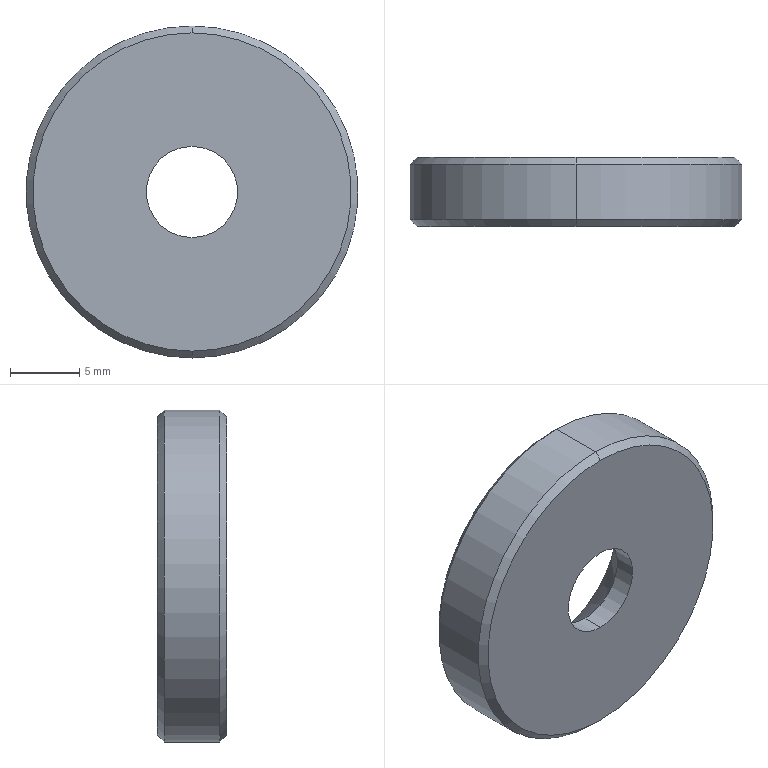Part | SolidWorks | features Chamfer 1, Extrusion 1, HoleWzd 1 | 1 solid | 12 faces | box 24 x 5 x 24 mm | volume 1909 mm3 | cone 6 | cylinder 4 | plane 2 | commonest cylinder face diameters 6.6 x2 24 x2
STEP:
#1=CARTESIAN_POINT('',(0.,5.,11.5));
#2=VERTEX_POINT('',#1);
#3=CARTESIAN_POINT('',(0.,5.,-11.5));
#4=VERTEX_POINT('',#3);
#5=CARTESIAN_POINT('',(0.,5.,0.));
#6=DIRECTION('',(0.,1.,0.));
#7=DIRECTION('',(0.,0.,1.));
#8=AXIS2_PLACEMENT_3D('',#5,#6,#7);
#9=CIRCLE('',#8,11.5);
#10=EDGE_CURVE('',#2,#4,#9,.T.);
#11=ORIENTED_EDGE('',*,*,#10,.F.);
#12=CARTESIAN_POINT('',(0.,4.5,12.));
#13=VERTEX_POINT('',#12);
#14=CARTESIAN_POINT('',(0.,5.,11.5));
#15=DIRECTION('',(0.,-0.7071,0.7071));
#16=VECTOR('',#15,1000.);
#17=LINE('',#14,#16);
#18=EDGE_CURVE('',#2,#13,#17,.T.);
#19=ORIENTED_EDGE('',*,*,#18,.T.);
#20=CARTESIAN_POINT('',(0.,4.5,-12.));
#21=VERTEX_POINT('',#20);
#22=CARTESIAN_POINT('',(0.,4.5,0.));
#23=DIRECTION('',(0.,-1.,0.));
#24=DIRECTION('',(0.,0.,1.));
#25=AXIS2_PLACEMENT_3D('',#22,#23,#24);
#26=CIRCLE('',#25,12.);
#27=EDGE_CURVE('',#21,#13,#26,.T.);
#28=ORIENTED_EDGE('',*,*,#27,.F.);
#29=CARTESIAN_POINT('',(0.,5.,-11.5));
#30=DIRECTION('',(0.,-0.7071,-0.7071));
#31=VECTOR('',#30,1000.);
#32=LINE('',#29,#31);
#33=EDGE_CURVE('',#4,#21,#32,.T.);
#34=ORIENTED_EDGE('',*,*,#33,.F.);
#35=EDGE_LOOP('',(#11,#19,#28,#34));
#36=FACE_OUTER_BOUND('',#35,.T.);
#37=CARTESIAN_POINT('',(0.,5.,0.));
#38=DIRECTION('',(0.,-1.,0.));
#39=DIRECTION('',(0.,0.,-1.));
#40=AXIS2_PLACEMENT_3D('',#37,#38,#39);
#41=CONICAL_SURFACE('',#40,11.5,0.7854);
#42=ADVANCED_FACE('',(#36),#41,.T.);
#43=CARTESIAN_POINT('',(0.,0.,-11.5));
#44=VERTEX_POINT('',#43);
#45=CARTESIAN_POINT('',(0.,0.,11.5));
#46=VERTEX_POINT('',#45);
#47=CARTESIAN_POINT('',(0.,0.,0.));
#48=DIRECTION('',(0.,-1.,0.));
#49=DIRECTION('',(0.,0.,1.));
#50=AXIS2_PLACEMENT_3D('',#47,#48,#49);
#51=CIRCLE('',#50,11.5);
#52=EDGE_CURVE('',#44,#46,#51,.T.);
#53=ORIENTED_EDGE('',*,*,#52,.F.);
#54=CARTESIAN_POINT('',(0.,0.5,-12.));
#55=VERTEX_POINT('',#54);
#56=CARTESIAN_POINT('',(0.,0.5,-12.));
#57=DIRECTION('',(0.,0.7071,-0.7071));
#58=VECTOR('',#57,1000.);
#59=LINE('',#56,#58);
#60=EDGE_CURVE('',#44,#55,#59,.T.);
#61=ORIENTED_EDGE('',*,*,#60,.T.);
#62=CARTESIAN_POINT('',(0.,0.5,12.));
#63=VERTEX_POINT('',#62);
#64=CARTESIAN_POINT('',(0.,0.5,0.));
#65=DIRECTION('',(0.,1.,0.));
#66=DIRECTION('',(0.,0.,1.));
#67=AXIS2_PLACEMENT_3D('',#64,#65,#66);
#68=CIRCLE('',#67,12.);
#69=EDGE_CURVE('',#63,#55,#68,.T.);
#70=ORIENTED_EDGE('',*,*,#69,.F.);
#71=CARTESIAN_POINT('',(0.,0.5,12.));
#72=DIRECTION('',(0.,0.7071,0.7071));
#73=VECTOR('',#72,1000.);
#74=LINE('',#71,#73);
#75=EDGE_CURVE('',#46,#63,#74,.T.);
#76=ORIENTED_EDGE('',*,*,#75,.F.);
#77=EDGE_LOOP('',(#53,#61,#70,#76));
#78=FACE_OUTER_BOUND('',#77,.T.);
#79=CARTESIAN_POINT('',(0.,0.5,0.));
#80=DIRECTION('',(0.,1.,0.));
#81=DIRECTION('',(0.,0.,1.));
#82=AXIS2_PLACEMENT_3D('',#79,#80,#81);
#83=CONICAL_SURFACE('',#82,12.,0.7854);
#84=ADVANCED_FACE('',(#78),#83,.T.);
#85=CARTESIAN_POINT('',(0.,1.58,-3.3));
#86=VERTEX_POINT('',#85);
#87=CARTESIAN_POINT('',(0.,1.58,3.3));
#88=VERTEX_POINT('',#87);
#89=CARTESIAN_POINT('',(0.,1.58,0.));
#90=DIRECTION('',(0.,1.,0.));
#91=DIRECTION('',(0.,0.,1.));
#92=AXIS2_PLACEMENT_3D('',#89,#90,#91);
#93=CIRCLE('',#92,3.3);
#94=EDGE_CURVE('',#86,#88,#93,.T.);
#95=ORIENTED_EDGE('',*,*,#94,.F.);
#96=CARTESIAN_POINT('',(0.,5.,-6.72));
#97=VERTEX_POINT('',#96);
#98=CARTESIAN_POINT('',(0.,5.,-6.72));
#99=DIRECTION('',(0.,0.7071,-0.7071));
#100=VECTOR('',#99,1000.);
#101=LINE('',#98,#100);
#102=EDGE_CURVE('',#86,#97,#101,.T.);
#103=ORIENTED_EDGE('',*,*,#102,.T.);
#104=CARTESIAN_POINT('',(0.,5.,6.72));
#105=VERTEX_POINT('',#104);
#106=CARTESIAN_POINT('',(0.,5.,0.));
#107=DIRECTION('',(0.,1.,0.));
#108=DIRECTION('',(0.,0.,1.));
#109=AXIS2_PLACEMENT_3D('',#106,#107,#108);
#110=CIRCLE('',#109,6.72);
#111=EDGE_CURVE('',#97,#105,#110,.T.);
#112=ORIENTED_EDGE('',*,*,#111,.T.);
#113=CARTESIAN_POINT('',(0.,5.,6.72));
#114=DIRECTION('',(0.,0.7071,0.7071));
#115=VECTOR('',#114,1000.);
#116=LINE('',#113,#115);
#117=EDGE_CURVE('',#88,#105,#116,.T.);
#118=ORIENTED_EDGE('',*,*,#117,.F.);
#119=EDGE_LOOP('',(#95,#103,#112,#118));
#120=FACE_OUTER_BOUND('',#119,.T.);
#121=CARTESIAN_POINT('',(0.,5.,0.));
#122=DIRECTION('',(0.,1.,0.));
#123=DIRECTION('',(0.,0.,1.));
#124=AXIS2_PLACEMENT_3D('',#121,#122,#123);
#125=CONICAL_SURFACE('',#124,6.72,0.7854);
#126=ADVANCED_FACE('',(#120),#125,.F.);
#127=CARTESIAN_POINT('',(0.,0.,-3.3));
#128=VERTEX_POINT('',#127);
#129=CARTESIAN_POINT('',(0.,0.,3.3));
#130=VERTEX_POINT('',#129);
#131=CARTESIAN_POINT('',(0.,0.,0.));
#132=DIRECTION('',(0.,1.,0.));
#133=DIRECTION('',(0.,0.,1.));
#134=AXIS2_PLACEMENT_3D('',#131,#132,#133);
#135=CIRCLE('',#134,3.3);
#136=EDGE_CURVE('',#128,#130,#135,.T.);
#137=ORIENTED_EDGE('',*,*,#136,.F.);
#138=CARTESIAN_POINT('',(0.,5.,-3.3));
#139=DIRECTION('',(0.,1.,0.));
#140=VECTOR('',#139,1000.);
#141=LINE('',#138,#140);
#142=EDGE_CURVE('',#128,#86,#141,.T.);
#143=ORIENTED_EDGE('',*,*,#142,.T.);
#144=ORIENTED_EDGE('',*,*,#94,.T.);
#145=CARTESIAN_POINT('',(0.,5.,3.3));
#146=DIRECTION('',(0.,1.,0.));
#147=VECTOR('',#146,1000.);
#148=LINE('',#145,#147);
#149=EDGE_CURVE('',#130,#88,#148,.T.);
#150=ORIENTED_EDGE('',*,*,#149,.F.);
#151=EDGE_LOOP('',(#137,#143,#144,#150));
#152=FACE_OUTER_BOUND('',#151,.T.);
#153=CARTESIAN_POINT('',(0.,5.,0.));
#154=DIRECTION('',(0.,1.,0.));
#155=DIRECTION('',(0.,0.,1.));
#156=AXIS2_PLACEMENT_3D('',#153,#154,#155);
#157=CYLINDRICAL_SURFACE('',#156,3.3);
#158=ADVANCED_FACE('',(#152),#157,.F.);
#159=ORIENTED_EDGE('',*,*,#27,.T.);
#160=CARTESIAN_POINT('',(0.,5.,12.));
#161=DIRECTION('',(0.,-1.,0.));
#162=VECTOR('',#161,1000.);
#163=LINE('',#160,#162);
#164=EDGE_CURVE('',#13,#63,#163,.T.);
#165=ORIENTED_EDGE('',*,*,#164,.T.);
#166=ORIENTED_EDGE('',*,*,#69,.T.);
#167=CARTESIAN_POINT('',(0.,5.,-12.));
#168=DIRECTION('',(0.,-1.,0.));
#169=VECTOR('',#168,1000.);
#170=LINE('',#167,#169);
#171=EDGE_CURVE('',#21,#55,#170,.T.);
#172=ORIENTED_EDGE('',*,*,#171,.F.);
#173=EDGE_LOOP('',(#159,#165,#166,#172));
#174=FACE_OUTER_BOUND('',#173,.T.);
#175=CARTESIAN_POINT('',(0.,5.,0.));
#176=DIRECTION('',(0.,-1.,0.));
#177=DIRECTION('',(0.,0.,-1.));
#178=AXIS2_PLACEMENT_3D('',#175,#176,#177);
#179=CYLINDRICAL_SURFACE('',#178,12.);
#180=ADVANCED_FACE('',(#174),#179,.T.);
#181=ORIENTED_EDGE('',*,*,#164,.F.);
#182=CARTESIAN_POINT('',(0.,4.5,0.));
#183=DIRECTION('',(0.,-1.,0.));
#184=DIRECTION('',(0.,0.,1.));
#185=AXIS2_PLACEMENT_3D('',#182,#183,#184);
#186=CIRCLE('',#185,12.);
#187=EDGE_CURVE('',#13,#21,#186,.T.);
#188=ORIENTED_EDGE('',*,*,#187,.T.);
#189=ORIENTED_EDGE('',*,*,#171,.T.);
#190=CARTESIAN_POINT('',(0.,0.5,0.));
#191=DIRECTION('',(0.,1.,0.));
#192=DIRECTION('',(0.,0.,1.));
#193=AXIS2_PLACEMENT_3D('',#190,#191,#192);
#194=CIRCLE('',#193,12.);
#195=EDGE_CURVE('',#55,#63,#194,.T.);
#196=ORIENTED_EDGE('',*,*,#195,.T.);
#197=EDGE_LOOP('',(#181,#188,#189,#196));
#198=FACE_OUTER_BOUND('',#197,.T.);
#199=CARTESIAN_POINT('',(0.,5.,0.));
#200=DIRECTION('',(0.,-1.,0.));
#201=DIRECTION('',(0.,0.,-1.));
#202=AXIS2_PLACEMENT_3D('',#199,#200,#201);
#203=CYLINDRICAL_SURFACE('',#202,12.);
#204=ADVANCED_FACE('',(#198),#203,.T.);
#205=CARTESIAN_POINT('',(0.,5.,0.));
#206=DIRECTION('',(0.,1.,0.));
#207=DIRECTION('',(0.,0.,1.));
#208=AXIS2_PLACEMENT_3D('',#205,#206,#207);
#209=CIRCLE('',#208,11.5);
#210=EDGE_CURVE('',#4,#2,#209,.T.);
#211=ORIENTED_EDGE('',*,*,#210,.T.);
#212=ORIENTED_EDGE('',*,*,#10,.T.);
#213=EDGE_LOOP('',(#211,#212));
#214=FACE_OUTER_BOUND('',#213,.T.);
#215=CARTESIAN_POINT('',(0.,5.,0.));
#216=DIRECTION('',(0.,1.,0.));
#217=DIRECTION('',(0.,0.,1.));
#218=AXIS2_PLACEMENT_3D('',#215,#216,#217);
#219=CIRCLE('',#218,6.72);
#220=EDGE_CURVE('',#105,#97,#219,.T.);
#221=ORIENTED_EDGE('',*,*,#220,.F.);
#222=ORIENTED_EDGE('',*,*,#111,.F.);
#223=EDGE_LOOP('',(#221,#222));
#224=FACE_BOUND('',#223,.T.);
#225=CARTESIAN_POINT('',(0.,5.,0.));
#226=DIRECTION('',(0.,1.,0.));
#227=DIRECTION('',(0.,0.,1.));
#228=AXIS2_PLACEMENT_3D('',#225,#226,#227);
#229=PLANE('',#228);
#230=ADVANCED_FACE('',(#214,#224),#229,.T.);
#231=CARTESIAN_POINT('',(0.,0.,0.));
#232=DIRECTION('',(0.,-1.,0.));
#233=DIRECTION('',(0.,0.,1.));
#234=AXIS2_PLACEMENT_3D('',#231,#232,#233);
#235=CIRCLE('',#234,11.5);
#236=EDGE_CURVE('',#46,#44,#235,.T.);
#237=ORIENTED_EDGE('',*,*,#236,.T.);
#238=ORIENTED_EDGE('',*,*,#52,.T.);
#239=EDGE_LOOP('',(#237,#238));
#240=FACE_OUTER_BOUND('',#239,.T.);
#241=CARTESIAN_POINT('',(0.,0.,0.));
#242=DIRECTION('',(0.,1.,0.));
#243=DIRECTION('',(0.,0.,1.));
#244=AXIS2_PLACEMENT_3D('',#241,#242,#243);
#245=CIRCLE('',#244,3.3);
#246=EDGE_CURVE('',#130,#128,#245,.T.);
#247=ORIENTED_EDGE('',*,*,#246,.T.);
#248=ORIENTED_EDGE('',*,*,#136,.T.);
#249=EDGE_LOOP('',(#247,#248));
#250=FACE_BOUND('',#249,.T.);
#251=CARTESIAN_POINT('',(0.,0.,0.));
#252=DIRECTION('',(0.,1.,0.));
#253=DIRECTION('',(0.,0.,1.));
#254=AXIS2_PLACEMENT_3D('',#251,#252,#253);
#255=PLANE('',#254);
#256=ADVANCED_FACE('',(#240,#250),#255,.F.);
#257=ORIENTED_EDGE('',*,*,#142,.F.);
#258=ORIENTED_EDGE('',*,*,#246,.F.);
#259=ORIENTED_EDGE('',*,*,#149,.T.);
#260=CARTESIAN_POINT('',(0.,1.58,0.));
#261=DIRECTION('',(0.,1.,0.));
#262=DIRECTION('',(0.,0.,1.));
#263=AXIS2_PLACEMENT_3D('',#260,#261,#262);
#264=CIRCLE('',#263,3.3);
#265=EDGE_CURVE('',#88,#86,#264,.T.);
#266=ORIENTED_EDGE('',*,*,#265,.T.);
#267=EDGE_LOOP('',(#257,#258,#259,#266));
#268=FACE_OUTER_BOUND('',#267,.T.);
#269=CARTESIAN_POINT('',(0.,5.,0.));
#270=DIRECTION('',(0.,1.,0.));
#271=DIRECTION('',(0.,0.,1.));
#272=AXIS2_PLACEMENT_3D('',#269,#270,#271);
#273=CYLINDRICAL_SURFACE('',#272,3.3);
#274=ADVANCED_FACE('',(#268),#273,.F.);
#275=ORIENTED_EDGE('',*,*,#102,.F.);
#276=ORIENTED_EDGE('',*,*,#265,.F.);
#277=ORIENTED_EDGE('',*,*,#117,.T.);
#278=ORIENTED_EDGE('',*,*,#220,.T.);
#279=EDGE_LOOP('',(#275,#276,#277,#278));
#280=FACE_OUTER_BOUND('',#279,.T.);
#281=CARTESIAN_POINT('',(0.,5.,0.));
#282=DIRECTION('',(0.,1.,0.));
#283=DIRECTION('',(0.,0.,1.));
#284=AXIS2_PLACEMENT_3D('',#281,#282,#283);
#285=CONICAL_SURFACE('',#284,6.72,0.7854);
#286=ADVANCED_FACE('',(#280),#285,.F.);
#287=ORIENTED_EDGE('',*,*,#60,.F.);
#288=ORIENTED_EDGE('',*,*,#236,.F.);
#289=ORIENTED_EDGE('',*,*,#75,.T.);
#290=ORIENTED_EDGE('',*,*,#195,.F.);
#291=EDGE_LOOP('',(#287,#288,#289,#290));
#292=FACE_OUTER_BOUND('',#291,.T.);
#293=CARTESIAN_POINT('',(0.,0.5,0.));
#294=DIRECTION('',(0.,1.,0.));
#295=DIRECTION('',(0.,0.,1.));
#296=AXIS2_PLACEMENT_3D('',#293,#294,#295);
#297=CONICAL_SURFACE('',#296,12.,0.7854);
#298=ADVANCED_FACE('',(#292),#297,.T.);
#299=ORIENTED_EDGE('',*,*,#18,.F.);
#300=ORIENTED_EDGE('',*,*,#210,.F.);
#301=ORIENTED_EDGE('',*,*,#33,.T.);
#302=ORIENTED_EDGE('',*,*,#187,.F.);
#303=EDGE_LOOP('',(#299,#300,#301,#302));
#304=FACE_OUTER_BOUND('',#303,.T.);
#305=CARTESIAN_POINT('',(0.,5.,0.));
#306=DIRECTION('',(0.,-1.,0.));
#307=DIRECTION('',(0.,0.,-1.));
#308=AXIS2_PLACEMENT_3D('',#305,#306,#307);
#309=CONICAL_SURFACE('',#308,11.5,0.7854);
#310=ADVANCED_FACE('',(#304),#309,.T.);
#311=CLOSED_SHELL('',(#42,#84,#126,#158,#180,#204,#230,#256,#274,#286,#298,#310));
#312=MANIFOLD_SOLID_BREP('',#311);
#313=CARTESIAN_POINT('',(0.,0.,0.));
#314=DIRECTION('',(0.,0.,1.));
#315=DIRECTION('',(1.,0.,0.));
#316=AXIS2_PLACEMENT_3D('',#313,#314,#315);
#317=(LENGTH_UNIT()NAMED_UNIT(*)SI_UNIT(.MILLI.,.METRE.));
#318=UNCERTAINTY_MEASURE_WITH_UNIT(LENGTH_MEASURE(0.00001),#317,'','');
#319=(NAMED_UNIT(*)PLANE_ANGLE_UNIT()SI_UNIT($,.RADIAN.));
#320=(NAMED_UNIT(*)SI_UNIT($,.STERADIAN.)SOLID_ANGLE_UNIT());
#321=(GEOMETRIC_REPRESENTATION_CONTEXT(3)GLOBAL_UNCERTAINTY_ASSIGNED_CONTEXT((#318))GLOBAL_UNIT_ASSIGNED_CONTEXT((#317,#319,#320))REPRESENTATION_CONTEXT('',''));
#322=ADVANCED_BREP_SHAPE_REPRESENTATION('',(#312,#316),#321);